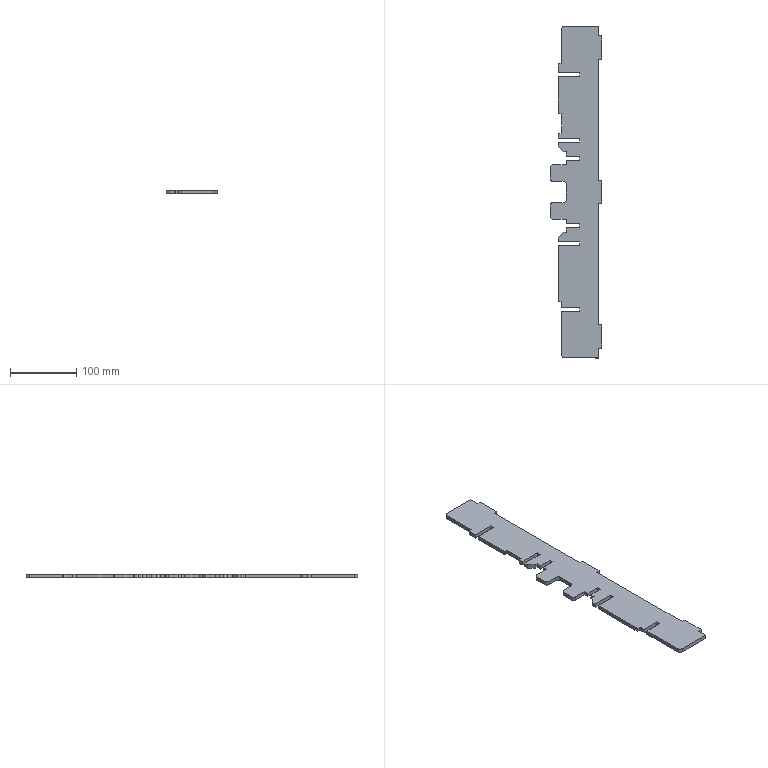Part | SolidWorks | features Fillet 1, FlatPattern 1, SMBaseFlange 1, SheetMetal 1 | 1 solid | 80 faces | box 78 x 500 x 6 mm | volume 170412 mm3 | plane 64 | cylinder 16 | commonest cylinder face diameters 2 x8 10 x8